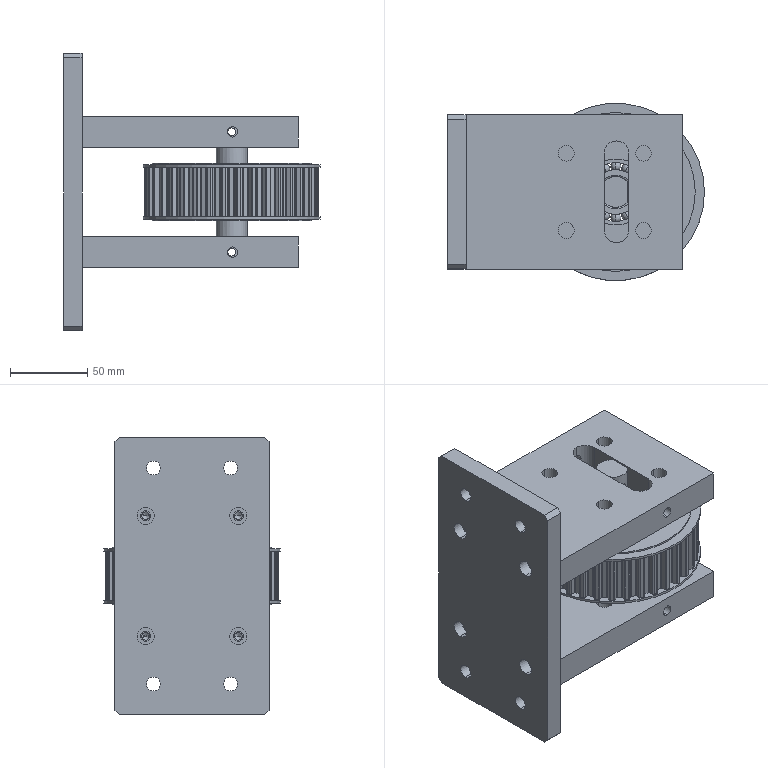Part | SolidWorks | features CompositeCurve 2 | 7 solids | 693 faces | box 166.5 x 115 x 180 mm | volume 1052923 mm3 | cylinder 330 | plane 169 | torus 106 | sphere 56 | cone 32 | commonest cylinder face diameters 1.6 x86 1.2 x84 112.74 x36 5 x20 10.2 x16 20 x10